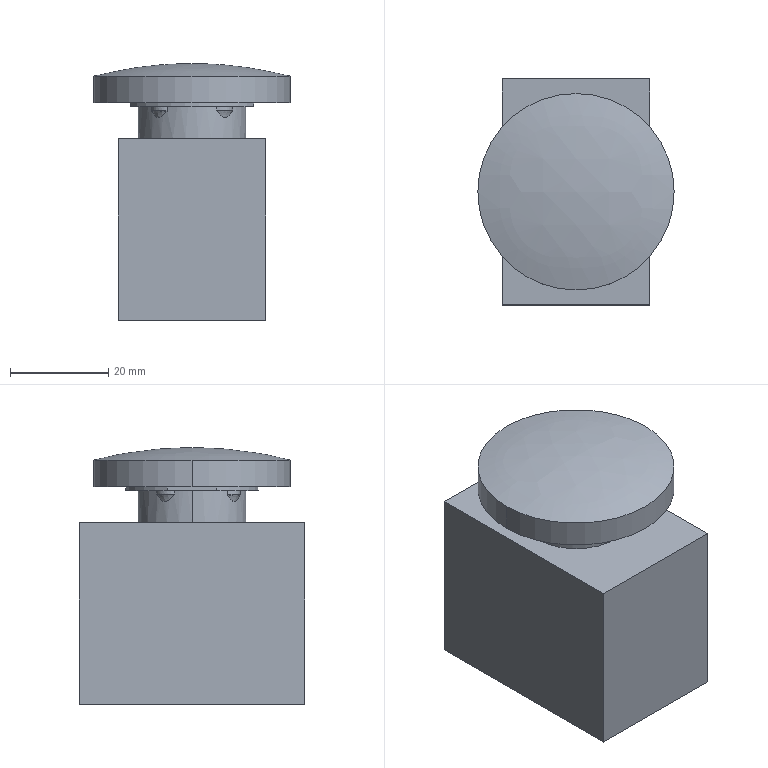Part | STEP file | ZBE-101-STOP-1_1 | 1 solid | 61 faces | box 40 x 46 x 52.3 mm | volume 62411 mm3 | plane 31 | cylinder 21 | spline 9 | commonest cylinder face diameters 4.8 x4 25.2 x4 6 x3 0.7 x2 22 x2 27.15 x2